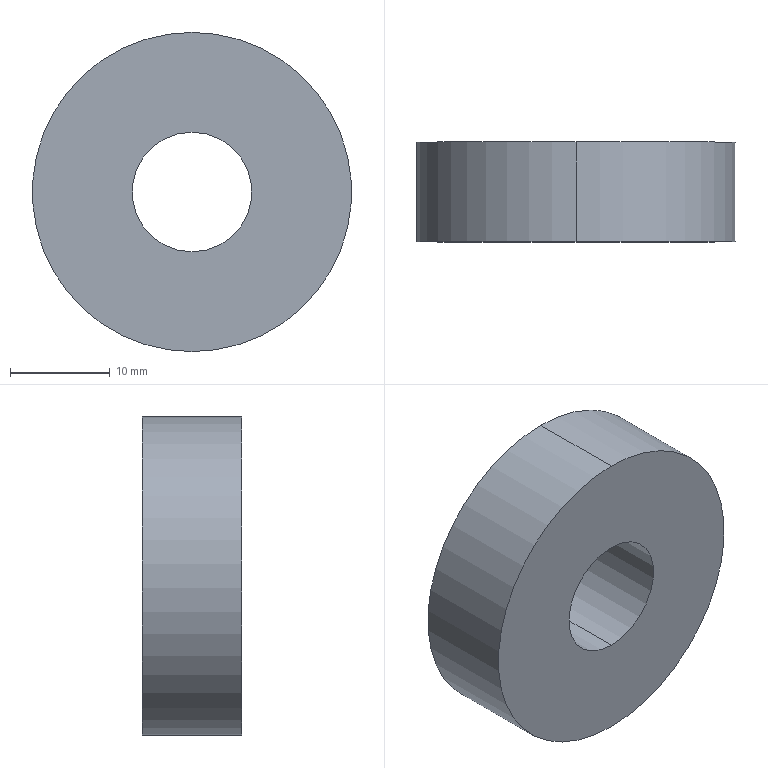Part | STEP file | SM140A-20-1140D-140A-600 Front bearing | 1 solid | 6 faces | box 32 x 10 x 32 mm | volume 6912 mm3 | cylinder 4 | plane 2 | commonest cylinder face diameters 12 x2 32 x2
STEP:
#1=CARTESIAN_POINT('',(0.,0.,0.));
#2=DIRECTION('',(0.,0.,1.));
#3=DIRECTION('',(1.,0.,0.));
#4=AXIS2_PLACEMENT_3D('',#1,#2,#3);
#5=CARTESIAN_POINT('',(0.,10.,-6.));
#6=VERTEX_POINT('',#5);
#7=CARTESIAN_POINT('',(0.,0.,-6.));
#8=VERTEX_POINT('',#7);
#9=CARTESIAN_POINT('',(0.,10.,-6.));
#10=DIRECTION('',(0.,-1.,0.));
#11=VECTOR('',#10,1.);
#12=LINE('',#9,#11);
#13=CARTESIAN_POINT('',(0.,10.,0.));
#14=DIRECTION('',(0.,-1.,0.));
#15=DIRECTION('',(0.,0.,-1.));
#16=AXIS2_PLACEMENT_3D('',#13,#14,#15);
#17=CYLINDRICAL_SURFACE('',#16,6.);
#18=CARTESIAN_POINT('',(6.283,0.));
#19=DIRECTION('',(0.,1.));
#20=VECTOR('',#19,1.);
#21=LINE('',#18,#20);
#22=(GEOMETRIC_REPRESENTATION_CONTEXT(2)PARAMETRIC_REPRESENTATION_CONTEXT()REPRESENTATION_CONTEXT('',''));
#23=DEFINITIONAL_REPRESENTATION('',(#21),#22);
#24=PCURVE('',#17,#23);
#25=CARTESIAN_POINT('',(0.,10.,0.));
#26=DIRECTION('',(0.,-1.,0.));
#27=DIRECTION('',(0.,0.,-1.));
#28=AXIS2_PLACEMENT_3D('',#25,#26,#27);
#29=CYLINDRICAL_SURFACE('',#28,6.);
#30=CARTESIAN_POINT('',(0.,0.));
#31=DIRECTION('',(0.,1.));
#32=VECTOR('',#31,1.);
#33=LINE('',#30,#32);
#34=(GEOMETRIC_REPRESENTATION_CONTEXT(2)PARAMETRIC_REPRESENTATION_CONTEXT()REPRESENTATION_CONTEXT('',''));
#35=DEFINITIONAL_REPRESENTATION('',(#33),#34);
#36=PCURVE('',#29,#35);
#37=SURFACE_CURVE('',#12,(#24,#36),.PCURVE_S1.);
#38=EDGE_CURVE('',#6,#8,#37,.T.);
#39=ORIENTED_EDGE('',*,*,#38,.T.);
#40=CARTESIAN_POINT('',(0.,0.,6.));
#41=VERTEX_POINT('',#40);
#42=CARTESIAN_POINT('',(0.,0.,0.));
#43=DIRECTION('',(0.,1.,0.));
#44=DIRECTION('',(0.,0.,1.));
#45=AXIS2_PLACEMENT_3D('',#42,#43,#44);
#46=CIRCLE('',#45,6.);
#47=CARTESIAN_POINT('',(9.425,10.));
#48=DIRECTION('',(-1.,0.));
#49=VECTOR('',#48,1.);
#50=LINE('',#47,#49);
#51=(GEOMETRIC_REPRESENTATION_CONTEXT(2)PARAMETRIC_REPRESENTATION_CONTEXT()REPRESENTATION_CONTEXT('',''));
#52=DEFINITIONAL_REPRESENTATION('',(#50),#51);
#53=PCURVE('',#17,#52);
#54=CARTESIAN_POINT('',(0.,0.,0.));
#55=DIRECTION('',(0.,1.,0.));
#56=DIRECTION('',(0.,0.,1.));
#57=AXIS2_PLACEMENT_3D('',#54,#55,#56);
#58=PLANE('',#57);
#59=CARTESIAN_POINT('',(0.,0.));
#60=DIRECTION('',(1.,0.));
#61=AXIS2_PLACEMENT_2D('',#59,#60);
#62=CIRCLE('',#61,6.);
#63=(GEOMETRIC_REPRESENTATION_CONTEXT(2)PARAMETRIC_REPRESENTATION_CONTEXT()REPRESENTATION_CONTEXT('',''));
#64=DEFINITIONAL_REPRESENTATION('',(#62),#63);
#65=PCURVE('',#58,#64);
#66=SURFACE_CURVE('',#46,(#53,#65),.PCURVE_S1.);
#67=EDGE_CURVE('',#8,#41,#66,.T.);
#68=ORIENTED_EDGE('',*,*,#67,.T.);
#69=CARTESIAN_POINT('',(0.,10.,6.));
#70=VERTEX_POINT('',#69);
#71=CARTESIAN_POINT('',(0.,10.,6.));
#72=DIRECTION('',(0.,-1.,0.));
#73=VECTOR('',#72,1.);
#74=LINE('',#71,#73);
#75=CARTESIAN_POINT('',(3.142,0.));
#76=DIRECTION('',(0.,1.));
#77=VECTOR('',#76,1.);
#78=LINE('',#75,#77);
#79=(GEOMETRIC_REPRESENTATION_CONTEXT(2)PARAMETRIC_REPRESENTATION_CONTEXT()REPRESENTATION_CONTEXT('',''));
#80=DEFINITIONAL_REPRESENTATION('',(#78),#79);
#81=PCURVE('',#17,#80);
#82=CARTESIAN_POINT('',(3.142,0.));
#83=DIRECTION('',(0.,1.));
#84=VECTOR('',#83,1.);
#85=LINE('',#82,#84);
#86=(GEOMETRIC_REPRESENTATION_CONTEXT(2)PARAMETRIC_REPRESENTATION_CONTEXT()REPRESENTATION_CONTEXT('',''));
#87=DEFINITIONAL_REPRESENTATION('',(#85),#86);
#88=PCURVE('',#29,#87);
#89=SURFACE_CURVE('',#74,(#81,#88),.PCURVE_S1.);
#90=EDGE_CURVE('',#70,#41,#89,.T.);
#91=ORIENTED_EDGE('',*,*,#90,.F.);
#92=CARTESIAN_POINT('',(0.,10.,0.));
#93=DIRECTION('',(0.,1.,0.));
#94=DIRECTION('',(0.,0.,1.));
#95=AXIS2_PLACEMENT_3D('',#92,#93,#94);
#96=CIRCLE('',#95,6.);
#97=CARTESIAN_POINT('',(9.425,0.));
#98=DIRECTION('',(-1.,0.));
#99=VECTOR('',#98,1.);
#100=LINE('',#97,#99);
#101=(GEOMETRIC_REPRESENTATION_CONTEXT(2)PARAMETRIC_REPRESENTATION_CONTEXT()REPRESENTATION_CONTEXT('',''));
#102=DEFINITIONAL_REPRESENTATION('',(#100),#101);
#103=PCURVE('',#17,#102);
#104=CARTESIAN_POINT('',(0.,10.,0.));
#105=DIRECTION('',(0.,1.,0.));
#106=DIRECTION('',(0.,0.,1.));
#107=AXIS2_PLACEMENT_3D('',#104,#105,#106);
#108=PLANE('',#107);
#109=CARTESIAN_POINT('',(0.,0.));
#110=DIRECTION('',(1.,0.));
#111=AXIS2_PLACEMENT_2D('',#109,#110);
#112=CIRCLE('',#111,6.);
#113=(GEOMETRIC_REPRESENTATION_CONTEXT(2)PARAMETRIC_REPRESENTATION_CONTEXT()REPRESENTATION_CONTEXT('',''));
#114=DEFINITIONAL_REPRESENTATION('',(#112),#113);
#115=PCURVE('',#108,#114);
#116=SURFACE_CURVE('',#96,(#103,#115),.PCURVE_S1.);
#117=EDGE_CURVE('',#6,#70,#116,.T.);
#118=ORIENTED_EDGE('',*,*,#117,.F.);
#119=EDGE_LOOP('',(#39,#68,#91,#118));
#120=FACE_BOUND('',#119,.F.);
#121=ADVANCED_FACE('',(#120),#17,.F.);
#122=CARTESIAN_POINT('',(0.,10.,16.));
#123=VERTEX_POINT('',#122);
#124=CARTESIAN_POINT('',(0.,10.,-16.));
#125=VERTEX_POINT('',#124);
#126=CARTESIAN_POINT('',(0.,10.,0.));
#127=DIRECTION('',(0.,1.,0.));
#128=DIRECTION('',(0.,0.,1.));
#129=AXIS2_PLACEMENT_3D('',#126,#127,#128);
#130=CIRCLE('',#129,16.);
#131=CARTESIAN_POINT('',(0.,10.,0.));
#132=DIRECTION('',(0.,-1.,0.));
#133=DIRECTION('',(0.,0.,-1.));
#134=AXIS2_PLACEMENT_3D('',#131,#132,#133);
#135=CYLINDRICAL_SURFACE('',#134,16.);
#136=CARTESIAN_POINT('',(3.142,0.));
#137=DIRECTION('',(-1.,0.));
#138=VECTOR('',#137,1.);
#139=LINE('',#136,#138);
#140=(GEOMETRIC_REPRESENTATION_CONTEXT(2)PARAMETRIC_REPRESENTATION_CONTEXT()REPRESENTATION_CONTEXT('',''));
#141=DEFINITIONAL_REPRESENTATION('',(#139),#140);
#142=PCURVE('',#135,#141);
#143=CARTESIAN_POINT('',(0.,0.));
#144=DIRECTION('',(1.,0.));
#145=AXIS2_PLACEMENT_2D('',#143,#144);
#146=CIRCLE('',#145,16.);
#147=(GEOMETRIC_REPRESENTATION_CONTEXT(2)PARAMETRIC_REPRESENTATION_CONTEXT()REPRESENTATION_CONTEXT('',''));
#148=DEFINITIONAL_REPRESENTATION('',(#146),#147);
#149=PCURVE('',#108,#148);
#150=SURFACE_CURVE('',#130,(#142,#149),.PCURVE_S1.);
#151=EDGE_CURVE('',#123,#125,#150,.T.);
#152=ORIENTED_EDGE('',*,*,#151,.F.);
#153=CARTESIAN_POINT('',(0.,0.,16.));
#154=VERTEX_POINT('',#153);
#155=CARTESIAN_POINT('',(0.,10.,16.));
#156=DIRECTION('',(0.,-1.,0.));
#157=VECTOR('',#156,1.);
#158=LINE('',#155,#157);
#159=CARTESIAN_POINT('',(3.142,0.));
#160=DIRECTION('',(0.,1.));
#161=VECTOR('',#160,1.);
#162=LINE('',#159,#161);
#163=(GEOMETRIC_REPRESENTATION_CONTEXT(2)PARAMETRIC_REPRESENTATION_CONTEXT()REPRESENTATION_CONTEXT('',''));
#164=DEFINITIONAL_REPRESENTATION('',(#162),#163);
#165=PCURVE('',#135,#164);
#166=CARTESIAN_POINT('',(0.,10.,0.));
#167=DIRECTION('',(0.,-1.,0.));
#168=DIRECTION('',(0.,0.,-1.));
#169=AXIS2_PLACEMENT_3D('',#166,#167,#168);
#170=CYLINDRICAL_SURFACE('',#169,16.);
#171=CARTESIAN_POINT('',(3.142,0.));
#172=DIRECTION('',(0.,1.));
#173=VECTOR('',#172,1.);
#174=LINE('',#171,#173);
#175=(GEOMETRIC_REPRESENTATION_CONTEXT(2)PARAMETRIC_REPRESENTATION_CONTEXT()REPRESENTATION_CONTEXT('',''));
#176=DEFINITIONAL_REPRESENTATION('',(#174),#175);
#177=PCURVE('',#170,#176);
#178=SURFACE_CURVE('',#158,(#165,#177),.PCURVE_S1.);
#179=EDGE_CURVE('',#123,#154,#178,.T.);
#180=ORIENTED_EDGE('',*,*,#179,.T.);
#181=CARTESIAN_POINT('',(0.,0.,-16.));
#182=VERTEX_POINT('',#181);
#183=CARTESIAN_POINT('',(0.,0.,0.));
#184=DIRECTION('',(0.,1.,0.));
#185=DIRECTION('',(0.,0.,1.));
#186=AXIS2_PLACEMENT_3D('',#183,#184,#185);
#187=CIRCLE('',#186,16.);
#188=CARTESIAN_POINT('',(3.142,10.));
#189=DIRECTION('',(-1.,0.));
#190=VECTOR('',#189,1.);
#191=LINE('',#188,#190);
#192=(GEOMETRIC_REPRESENTATION_CONTEXT(2)PARAMETRIC_REPRESENTATION_CONTEXT()REPRESENTATION_CONTEXT('',''));
#193=DEFINITIONAL_REPRESENTATION('',(#191),#192);
#194=PCURVE('',#135,#193);
#195=CARTESIAN_POINT('',(0.,0.));
#196=DIRECTION('',(1.,0.));
#197=AXIS2_PLACEMENT_2D('',#195,#196);
#198=CIRCLE('',#197,16.);
#199=(GEOMETRIC_REPRESENTATION_CONTEXT(2)PARAMETRIC_REPRESENTATION_CONTEXT()REPRESENTATION_CONTEXT('',''));
#200=DEFINITIONAL_REPRESENTATION('',(#198),#199);
#201=PCURVE('',#58,#200);
#202=SURFACE_CURVE('',#187,(#194,#201),.PCURVE_S1.);
#203=EDGE_CURVE('',#154,#182,#202,.T.);
#204=ORIENTED_EDGE('',*,*,#203,.T.);
#205=CARTESIAN_POINT('',(0.,10.,-16.));
#206=DIRECTION('',(0.,-1.,0.));
#207=VECTOR('',#206,1.);
#208=LINE('',#205,#207);
#209=CARTESIAN_POINT('',(0.,0.));
#210=DIRECTION('',(0.,1.));
#211=VECTOR('',#210,1.);
#212=LINE('',#209,#211);
#213=(GEOMETRIC_REPRESENTATION_CONTEXT(2)PARAMETRIC_REPRESENTATION_CONTEXT()REPRESENTATION_CONTEXT('',''));
#214=DEFINITIONAL_REPRESENTATION('',(#212),#213);
#215=PCURVE('',#135,#214);
#216=CARTESIAN_POINT('',(6.283,0.));
#217=DIRECTION('',(0.,1.));
#218=VECTOR('',#217,1.);
#219=LINE('',#216,#218);
#220=(GEOMETRIC_REPRESENTATION_CONTEXT(2)PARAMETRIC_REPRESENTATION_CONTEXT()REPRESENTATION_CONTEXT('',''));
#221=DEFINITIONAL_REPRESENTATION('',(#219),#220);
#222=PCURVE('',#170,#221);
#223=SURFACE_CURVE('',#208,(#215,#222),.PCURVE_S1.);
#224=EDGE_CURVE('',#125,#182,#223,.T.);
#225=ORIENTED_EDGE('',*,*,#224,.F.);
#226=EDGE_LOOP('',(#152,#180,#204,#225));
#227=FACE_BOUND('',#226,.T.);
#228=ADVANCED_FACE('',(#227),#135,.T.);
#229=CARTESIAN_POINT('',(0.,10.,0.));
#230=DIRECTION('',(0.,1.,0.));
#231=DIRECTION('',(0.,0.,1.));
#232=AXIS2_PLACEMENT_3D('',#229,#230,#231);
#233=CIRCLE('',#232,16.);
#234=CARTESIAN_POINT('',(0.,0.));
#235=DIRECTION('',(1.,0.));
#236=AXIS2_PLACEMENT_2D('',#234,#235);
#237=CIRCLE('',#236,16.);
#238=(GEOMETRIC_REPRESENTATION_CONTEXT(2)PARAMETRIC_REPRESENTATION_CONTEXT()REPRESENTATION_CONTEXT('',''));
#239=DEFINITIONAL_REPRESENTATION('',(#237),#238);
#240=PCURVE('',#108,#239);
#241=CARTESIAN_POINT('',(9.425,0.));
#242=DIRECTION('',(-1.,0.));
#243=VECTOR('',#242,1.);
#244=LINE('',#241,#243);
#245=(GEOMETRIC_REPRESENTATION_CONTEXT(2)PARAMETRIC_REPRESENTATION_CONTEXT()REPRESENTATION_CONTEXT('',''));
#246=DEFINITIONAL_REPRESENTATION('',(#244),#245);
#247=PCURVE('',#170,#246);
#248=SURFACE_CURVE('',#233,(#240,#247),.PCURVE_S1.);
#249=EDGE_CURVE('',#125,#123,#248,.T.);
#250=ORIENTED_EDGE('',*,*,#249,.T.);
#251=ORIENTED_EDGE('',*,*,#151,.T.);
#252=EDGE_LOOP('',(#250,#251));
#253=FACE_BOUND('',#252,.T.);
#254=ORIENTED_EDGE('',*,*,#117,.F.);
#255=CARTESIAN_POINT('',(0.,10.,0.));
#256=DIRECTION('',(0.,1.,0.));
#257=DIRECTION('',(0.,0.,1.));
#258=AXIS2_PLACEMENT_3D('',#255,#256,#257);
#259=CIRCLE('',#258,6.);
#260=CARTESIAN_POINT('',(0.,0.));
#261=DIRECTION('',(1.,0.));
#262=AXIS2_PLACEMENT_2D('',#260,#261);
#263=CIRCLE('',#262,6.);
#264=(GEOMETRIC_REPRESENTATION_CONTEXT(2)PARAMETRIC_REPRESENTATION_CONTEXT()REPRESENTATION_CONTEXT('',''));
#265=DEFINITIONAL_REPRESENTATION('',(#263),#264);
#266=PCURVE('',#108,#265);
#267=CARTESIAN_POINT('',(3.142,0.));
#268=DIRECTION('',(-1.,0.));
#269=VECTOR('',#268,1.);
#270=LINE('',#267,#269);
#271=(GEOMETRIC_REPRESENTATION_CONTEXT(2)PARAMETRIC_REPRESENTATION_CONTEXT()REPRESENTATION_CONTEXT('',''));
#272=DEFINITIONAL_REPRESENTATION('',(#270),#271);
#273=PCURVE('',#29,#272);
#274=SURFACE_CURVE('',#259,(#266,#273),.PCURVE_S1.);
#275=EDGE_CURVE('',#70,#6,#274,.T.);
#276=ORIENTED_EDGE('',*,*,#275,.F.);
#277=EDGE_LOOP('',(#254,#276));
#278=FACE_BOUND('',#277,.T.);
#279=ADVANCED_FACE('',(#253,#278),#108,.T.);
#280=CARTESIAN_POINT('',(0.,0.,0.));
#281=DIRECTION('',(0.,1.,0.));
#282=DIRECTION('',(0.,0.,1.));
#283=AXIS2_PLACEMENT_3D('',#280,#281,#282);
#284=CIRCLE('',#283,16.);
#285=CARTESIAN_POINT('',(0.,0.));
#286=DIRECTION('',(1.,0.));
#287=AXIS2_PLACEMENT_2D('',#285,#286);
#288=CIRCLE('',#287,16.);
#289=(GEOMETRIC_REPRESENTATION_CONTEXT(2)PARAMETRIC_REPRESENTATION_CONTEXT()REPRESENTATION_CONTEXT('',''));
#290=DEFINITIONAL_REPRESENTATION('',(#288),#289);
#291=PCURVE('',#58,#290);
#292=CARTESIAN_POINT('',(9.425,10.));
#293=DIRECTION('',(-1.,0.));
#294=VECTOR('',#293,1.);
#295=LINE('',#292,#294);
#296=(GEOMETRIC_REPRESENTATION_CONTEXT(2)PARAMETRIC_REPRESENTATION_CONTEXT()REPRESENTATION_CONTEXT('',''));
#297=DEFINITIONAL_REPRESENTATION('',(#295),#296);
#298=PCURVE('',#170,#297);
#299=SURFACE_CURVE('',#284,(#291,#298),.PCURVE_S1.);
#300=EDGE_CURVE('',#182,#154,#299,.T.);
#301=ORIENTED_EDGE('',*,*,#300,.F.);
#302=ORIENTED_EDGE('',*,*,#203,.F.);
#303=EDGE_LOOP('',(#301,#302));
#304=FACE_BOUND('',#303,.T.);
#305=ORIENTED_EDGE('',*,*,#67,.T.);
#306=CARTESIAN_POINT('',(0.,0.,0.));
#307=DIRECTION('',(0.,1.,0.));
#308=DIRECTION('',(0.,0.,1.));
#309=AXIS2_PLACEMENT_3D('',#306,#307,#308);
#310=CIRCLE('',#309,6.);
#311=CARTESIAN_POINT('',(0.,0.));
#312=DIRECTION('',(1.,0.));
#313=AXIS2_PLACEMENT_2D('',#311,#312);
#314=CIRCLE('',#313,6.);
#315=(GEOMETRIC_REPRESENTATION_CONTEXT(2)PARAMETRIC_REPRESENTATION_CONTEXT()REPRESENTATION_CONTEXT('',''));
#316=DEFINITIONAL_REPRESENTATION('',(#314),#315);
#317=PCURVE('',#58,#316);
#318=CARTESIAN_POINT('',(3.142,10.));
#319=DIRECTION('',(-1.,0.));
#320=VECTOR('',#319,1.);
#321=LINE('',#318,#320);
#322=(GEOMETRIC_REPRESENTATION_CONTEXT(2)PARAMETRIC_REPRESENTATION_CONTEXT()REPRESENTATION_CONTEXT('',''));
#323=DEFINITIONAL_REPRESENTATION('',(#321),#322);
#324=PCURVE('',#29,#323);
#325=SURFACE_CURVE('',#310,(#317,#324),.PCURVE_S1.);
#326=EDGE_CURVE('',#41,#8,#325,.T.);
#327=ORIENTED_EDGE('',*,*,#326,.T.);
#328=EDGE_LOOP('',(#305,#327));
#329=FACE_BOUND('',#328,.T.);
#330=ADVANCED_FACE('',(#304,#329),#58,.F.);
#331=ORIENTED_EDGE('',*,*,#179,.F.);
#332=ORIENTED_EDGE('',*,*,#249,.F.);
#333=ORIENTED_EDGE('',*,*,#224,.T.);
#334=ORIENTED_EDGE('',*,*,#300,.T.);
#335=EDGE_LOOP('',(#331,#332,#333,#334));
#336=FACE_BOUND('',#335,.T.);
#337=ADVANCED_FACE('',(#336),#170,.T.);
#338=ORIENTED_EDGE('',*,*,#326,.T.);
#339=ORIENTED_EDGE('',*,*,#38,.F.);
#340=ORIENTED_EDGE('',*,*,#275,.F.);
#341=ORIENTED_EDGE('',*,*,#90,.T.);
#342=EDGE_LOOP('',(#338,#339,#340,#341));
#343=FACE_BOUND('',#342,.F.);
#344=ADVANCED_FACE('',(#343),#29,.F.);
#345=CLOSED_SHELL('',(#121,#228,#279,#330,#337,#344));
#346=MANIFOLD_SOLID_BREP('',#345);
#347=(LENGTH_UNIT()NAMED_UNIT(*)SI_UNIT(.MILLI.,.METRE.));
#348=UNCERTAINTY_MEASURE_WITH_UNIT(LENGTH_MEASURE(0.0000001),#347,'','');
#349=(NAMED_UNIT(*)PLANE_ANGLE_UNIT()SI_UNIT($,.RADIAN.));
#350=(NAMED_UNIT(*)SI_UNIT($,.STERADIAN.)SOLID_ANGLE_UNIT());
#351=(GEOMETRIC_REPRESENTATION_CONTEXT(3)GLOBAL_UNCERTAINTY_ASSIGNED_CONTEXT((#348))GLOBAL_UNIT_ASSIGNED_CONTEXT((#347,#349,#350))REPRESENTATION_CONTEXT('',''));
#352=ADVANCED_BREP_SHAPE_REPRESENTATION('',(#4,#346),#351);